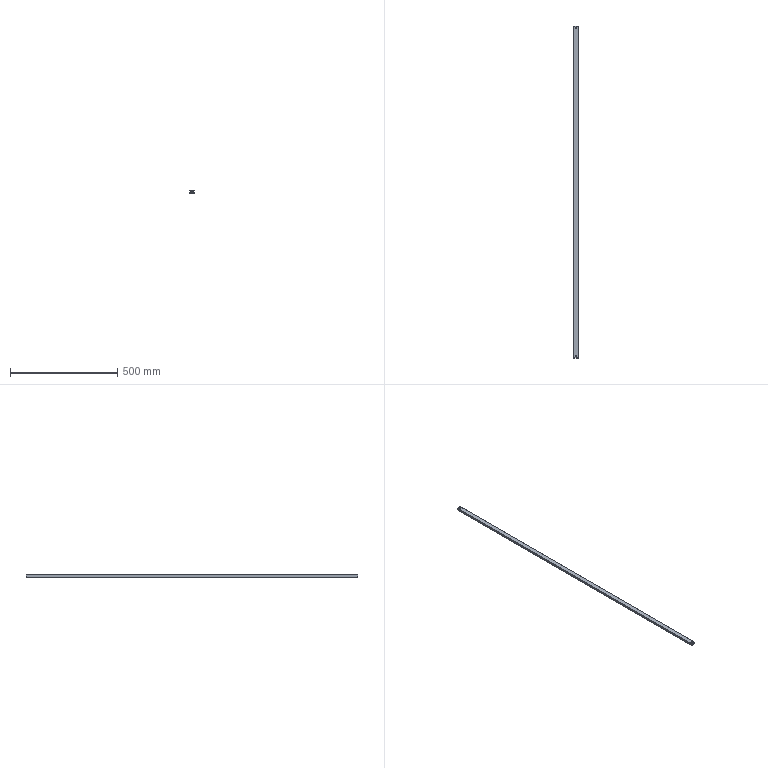Part | SolidWorks | features Extrusion 1, HoleWzd 1, WeldmentFeature 1 | 1 solid | 18 faces | box 20 x 1546 x 10 mm | volume 86388 mm3 | plane 10 | cylinder 8 | commonest cylinder face diameters 5.5 x4 10 x4
STEP:
#1=CARTESIAN_POINT('',(-5.,1538.3,-4.));
#2=VERTEX_POINT('',#1);
#3=CARTESIAN_POINT('',(5.,1538.3,-4.));
#4=VERTEX_POINT('',#3);
#5=CARTESIAN_POINT('',(0.,1538.3,-4.));
#6=DIRECTION('',(0.,0.,1.));
#7=DIRECTION('',(1.,0.,0.));
#8=AXIS2_PLACEMENT_3D('',#5,#6,#7);
#9=CIRCLE('',#8,5.);
#10=EDGE_CURVE('',#2,#4,#9,.T.);
#11=ORIENTED_EDGE('',*,*,#10,.T.);
#12=CARTESIAN_POINT('',(5.,1538.3,-5.));
#13=VERTEX_POINT('',#12);
#14=CARTESIAN_POINT('',(5.,1538.3,-5.));
#15=DIRECTION('',(0.,0.,-1.));
#16=VECTOR('',#15,1000.);
#17=LINE('',#14,#16);
#18=EDGE_CURVE('',#4,#13,#17,.T.);
#19=ORIENTED_EDGE('',*,*,#18,.T.);
#20=CARTESIAN_POINT('',(-5.,1538.3,-5.));
#21=VERTEX_POINT('',#20);
#22=CARTESIAN_POINT('',(0.,1538.3,-5.));
#23=DIRECTION('',(0.,0.,-1.));
#24=DIRECTION('',(-1.,0.,0.));
#25=AXIS2_PLACEMENT_3D('',#22,#23,#24);
#26=CIRCLE('',#25,5.);
#27=EDGE_CURVE('',#13,#21,#26,.T.);
#28=ORIENTED_EDGE('',*,*,#27,.T.);
#29=CARTESIAN_POINT('',(-5.,1538.3,-5.));
#30=DIRECTION('',(0.,0.,-1.));
#31=VECTOR('',#30,1000.);
#32=LINE('',#29,#31);
#33=EDGE_CURVE('',#2,#21,#32,.T.);
#34=ORIENTED_EDGE('',*,*,#33,.F.);
#35=EDGE_LOOP('',(#11,#19,#28,#34));
#36=FACE_OUTER_BOUND('',#35,.T.);
#37=CARTESIAN_POINT('',(0.,1538.3,-5.));
#38=DIRECTION('',(0.,0.,-1.));
#39=DIRECTION('',(-1.,0.,0.));
#40=AXIS2_PLACEMENT_3D('',#37,#38,#39);
#41=CYLINDRICAL_SURFACE('',#40,5.);
#42=ADVANCED_FACE('',(#36),#41,.F.);
#43=CARTESIAN_POINT('',(2.75,1538.3,5.));
#44=VERTEX_POINT('',#43);
#45=CARTESIAN_POINT('',(-2.75,1538.3,5.));
#46=VERTEX_POINT('',#45);
#47=CARTESIAN_POINT('',(0.,1538.3,5.));
#48=DIRECTION('',(0.,0.,-1.));
#49=DIRECTION('',(-1.,0.,0.));
#50=AXIS2_PLACEMENT_3D('',#47,#48,#49);
#51=CIRCLE('',#50,2.75);
#52=EDGE_CURVE('',#44,#46,#51,.T.);
#53=ORIENTED_EDGE('',*,*,#52,.F.);
#54=CARTESIAN_POINT('',(2.75,1538.3,4.));
#55=VERTEX_POINT('',#54);
#56=CARTESIAN_POINT('',(2.75,1538.3,-5.));
#57=DIRECTION('',(0.,0.,-1.));
#58=VECTOR('',#57,1000.);
#59=LINE('',#56,#58);
#60=EDGE_CURVE('',#44,#55,#59,.T.);
#61=ORIENTED_EDGE('',*,*,#60,.T.);
#62=CARTESIAN_POINT('',(-2.75,1538.3,4.));
#63=VERTEX_POINT('',#62);
#64=CARTESIAN_POINT('',(0.,1538.3,4.));
#65=DIRECTION('',(0.,0.,-1.));
#66=DIRECTION('',(-1.,0.,0.));
#67=AXIS2_PLACEMENT_3D('',#64,#65,#66);
#68=CIRCLE('',#67,2.75);
#69=EDGE_CURVE('',#55,#63,#68,.T.);
#70=ORIENTED_EDGE('',*,*,#69,.T.);
#71=CARTESIAN_POINT('',(-2.75,1538.3,-5.));
#72=DIRECTION('',(0.,0.,-1.));
#73=VECTOR('',#72,1000.);
#74=LINE('',#71,#73);
#75=EDGE_CURVE('',#46,#63,#74,.T.);
#76=ORIENTED_EDGE('',*,*,#75,.F.);
#77=EDGE_LOOP('',(#53,#61,#70,#76));
#78=FACE_OUTER_BOUND('',#77,.T.);
#79=CARTESIAN_POINT('',(0.,1538.3,-5.));
#80=DIRECTION('',(0.,0.,-1.));
#81=DIRECTION('',(-1.,0.,0.));
#82=AXIS2_PLACEMENT_3D('',#79,#80,#81);
#83=CYLINDRICAL_SURFACE('',#82,2.75);
#84=ADVANCED_FACE('',(#78),#83,.F.);
#85=CARTESIAN_POINT('',(2.75,8.,5.));
#86=VERTEX_POINT('',#85);
#87=CARTESIAN_POINT('',(-2.75,8.,5.));
#88=VERTEX_POINT('',#87);
#89=CARTESIAN_POINT('',(0.,8.,5.));
#90=DIRECTION('',(0.,0.,-1.));
#91=DIRECTION('',(-1.,0.,0.));
#92=AXIS2_PLACEMENT_3D('',#89,#90,#91);
#93=CIRCLE('',#92,2.75);
#94=EDGE_CURVE('',#86,#88,#93,.T.);
#95=ORIENTED_EDGE('',*,*,#94,.F.);
#96=CARTESIAN_POINT('',(2.75,8.,4.));
#97=VERTEX_POINT('',#96);
#98=CARTESIAN_POINT('',(2.75,8.,-5.));
#99=DIRECTION('',(0.,0.,-1.));
#100=VECTOR('',#99,1000.);
#101=LINE('',#98,#100);
#102=EDGE_CURVE('',#86,#97,#101,.T.);
#103=ORIENTED_EDGE('',*,*,#102,.T.);
#104=CARTESIAN_POINT('',(-2.75,8.,4.));
#105=VERTEX_POINT('',#104);
#106=CARTESIAN_POINT('',(0.,8.,4.));
#107=DIRECTION('',(0.,0.,-1.));
#108=DIRECTION('',(-1.,0.,0.));
#109=AXIS2_PLACEMENT_3D('',#106,#107,#108);
#110=CIRCLE('',#109,2.75);
#111=EDGE_CURVE('',#97,#105,#110,.T.);
#112=ORIENTED_EDGE('',*,*,#111,.T.);
#113=CARTESIAN_POINT('',(-2.75,8.,-5.));
#114=DIRECTION('',(0.,0.,-1.));
#115=VECTOR('',#114,1000.);
#116=LINE('',#113,#115);
#117=EDGE_CURVE('',#88,#105,#116,.T.);
#118=ORIENTED_EDGE('',*,*,#117,.F.);
#119=EDGE_LOOP('',(#95,#103,#112,#118));
#120=FACE_OUTER_BOUND('',#119,.T.);
#121=CARTESIAN_POINT('',(0.,8.,-5.));
#122=DIRECTION('',(0.,0.,-1.));
#123=DIRECTION('',(-1.,0.,0.));
#124=AXIS2_PLACEMENT_3D('',#121,#122,#123);
#125=CYLINDRICAL_SURFACE('',#124,2.75);
#126=ADVANCED_FACE('',(#120),#125,.F.);
#127=CARTESIAN_POINT('',(-5.,8.,-4.));
#128=VERTEX_POINT('',#127);
#129=CARTESIAN_POINT('',(5.,8.,-4.));
#130=VERTEX_POINT('',#129);
#131=CARTESIAN_POINT('',(0.,8.,-4.));
#132=DIRECTION('',(0.,0.,1.));
#133=DIRECTION('',(1.,0.,0.));
#134=AXIS2_PLACEMENT_3D('',#131,#132,#133);
#135=CIRCLE('',#134,5.);
#136=EDGE_CURVE('',#128,#130,#135,.T.);
#137=ORIENTED_EDGE('',*,*,#136,.T.);
#138=CARTESIAN_POINT('',(5.,8.,-5.));
#139=VERTEX_POINT('',#138);
#140=CARTESIAN_POINT('',(5.,8.,-5.));
#141=DIRECTION('',(0.,0.,-1.));
#142=VECTOR('',#141,1000.);
#143=LINE('',#140,#142);
#144=EDGE_CURVE('',#130,#139,#143,.T.);
#145=ORIENTED_EDGE('',*,*,#144,.T.);
#146=CARTESIAN_POINT('',(-5.,8.,-5.));
#147=VERTEX_POINT('',#146);
#148=CARTESIAN_POINT('',(0.,8.,-5.));
#149=DIRECTION('',(0.,0.,-1.));
#150=DIRECTION('',(-1.,0.,0.));
#151=AXIS2_PLACEMENT_3D('',#148,#149,#150);
#152=CIRCLE('',#151,5.);
#153=EDGE_CURVE('',#139,#147,#152,.T.);
#154=ORIENTED_EDGE('',*,*,#153,.T.);
#155=CARTESIAN_POINT('',(-5.,8.,-5.));
#156=DIRECTION('',(0.,0.,-1.));
#157=VECTOR('',#156,1000.);
#158=LINE('',#155,#157);
#159=EDGE_CURVE('',#128,#147,#158,.T.);
#160=ORIENTED_EDGE('',*,*,#159,.F.);
#161=EDGE_LOOP('',(#137,#145,#154,#160));
#162=FACE_OUTER_BOUND('',#161,.T.);
#163=CARTESIAN_POINT('',(0.,8.,-5.));
#164=DIRECTION('',(0.,0.,-1.));
#165=DIRECTION('',(-1.,0.,0.));
#166=AXIS2_PLACEMENT_3D('',#163,#164,#165);
#167=CYLINDRICAL_SURFACE('',#166,5.);
#168=ADVANCED_FACE('',(#162),#167,.F.);
#169=CARTESIAN_POINT('',(10.,1546.3,5.));
#170=VERTEX_POINT('',#169);
#171=CARTESIAN_POINT('',(10.,1546.3,-5.));
#172=VERTEX_POINT('',#171);
#173=CARTESIAN_POINT('',(10.,1546.3,-5.));
#174=DIRECTION('',(0.,0.,-1.));
#175=VECTOR('',#174,1000.);
#176=LINE('',#173,#175);
#177=EDGE_CURVE('',#170,#172,#176,.T.);
#178=ORIENTED_EDGE('',*,*,#177,.T.);
#179=CARTESIAN_POINT('',(-10.,1546.3,-5.));
#180=VERTEX_POINT('',#179);
#181=CARTESIAN_POINT('',(-10.,1546.3,-5.));
#182=DIRECTION('',(-1.,0.,0.));
#183=VECTOR('',#182,1000.);
#184=LINE('',#181,#183);
#185=EDGE_CURVE('',#172,#180,#184,.T.);
#186=ORIENTED_EDGE('',*,*,#185,.T.);
#187=CARTESIAN_POINT('',(-10.,1546.3,5.));
#188=VERTEX_POINT('',#187);
#189=CARTESIAN_POINT('',(-10.,1546.3,-5.));
#190=DIRECTION('',(0.,0.,1.));
#191=VECTOR('',#190,1000.);
#192=LINE('',#189,#191);
#193=EDGE_CURVE('',#180,#188,#192,.T.);
#194=ORIENTED_EDGE('',*,*,#193,.T.);
#195=CARTESIAN_POINT('',(-10.,1546.3,5.));
#196=DIRECTION('',(1.,0.,0.));
#197=VECTOR('',#196,1000.);
#198=LINE('',#195,#197);
#199=EDGE_CURVE('',#188,#170,#198,.T.);
#200=ORIENTED_EDGE('',*,*,#199,.T.);
#201=EDGE_LOOP('',(#178,#186,#194,#200));
#202=FACE_OUTER_BOUND('',#201,.T.);
#203=CARTESIAN_POINT('',(-9.,1546.3,-4.));
#204=VERTEX_POINT('',#203);
#205=CARTESIAN_POINT('',(-9.,1546.3,4.));
#206=VERTEX_POINT('',#205);
#207=CARTESIAN_POINT('',(-9.,1546.3,-4.));
#208=DIRECTION('',(0.,0.,1.));
#209=VECTOR('',#208,1000.);
#210=LINE('',#207,#209);
#211=EDGE_CURVE('',#204,#206,#210,.T.);
#212=ORIENTED_EDGE('',*,*,#211,.F.);
#213=CARTESIAN_POINT('',(9.,1546.3,-4.));
#214=VERTEX_POINT('',#213);
#215=CARTESIAN_POINT('',(-9.,1546.3,-4.));
#216=DIRECTION('',(-1.,0.,0.));
#217=VECTOR('',#216,1000.);
#218=LINE('',#215,#217);
#219=EDGE_CURVE('',#214,#204,#218,.T.);
#220=ORIENTED_EDGE('',*,*,#219,.F.);
#221=CARTESIAN_POINT('',(9.,1546.3,4.));
#222=VERTEX_POINT('',#221);
#223=CARTESIAN_POINT('',(9.,1546.3,-4.));
#224=DIRECTION('',(0.,0.,-1.));
#225=VECTOR('',#224,1000.);
#226=LINE('',#223,#225);
#227=EDGE_CURVE('',#222,#214,#226,.T.);
#228=ORIENTED_EDGE('',*,*,#227,.F.);
#229=CARTESIAN_POINT('',(-9.,1546.3,4.));
#230=DIRECTION('',(1.,0.,0.));
#231=VECTOR('',#230,1000.);
#232=LINE('',#229,#231);
#233=EDGE_CURVE('',#206,#222,#232,.T.);
#234=ORIENTED_EDGE('',*,*,#233,.F.);
#235=EDGE_LOOP('',(#212,#220,#228,#234));
#236=FACE_BOUND('',#235,.T.);
#237=CARTESIAN_POINT('',(0.,1546.3,0.));
#238=DIRECTION('',(0.,1.,0.));
#239=DIRECTION('',(0.,0.,1.));
#240=AXIS2_PLACEMENT_3D('',#237,#238,#239);
#241=PLANE('',#240);
#242=ADVANCED_FACE('',(#202,#236),#241,.T.);
#243=CARTESIAN_POINT('',(10.,0.,5.));
#244=VERTEX_POINT('',#243);
#245=CARTESIAN_POINT('',(10.,0.,-5.));
#246=VERTEX_POINT('',#245);
#247=CARTESIAN_POINT('',(10.,0.,-5.));
#248=DIRECTION('',(0.,0.,-1.));
#249=VECTOR('',#248,1000.);
#250=LINE('',#247,#249);
#251=EDGE_CURVE('',#244,#246,#250,.T.);
#252=ORIENTED_EDGE('',*,*,#251,.F.);
#253=CARTESIAN_POINT('',(-10.,0.,5.));
#254=VERTEX_POINT('',#253);
#255=CARTESIAN_POINT('',(-10.,0.,5.));
#256=DIRECTION('',(1.,0.,0.));
#257=VECTOR('',#256,1000.);
#258=LINE('',#255,#257);
#259=EDGE_CURVE('',#254,#244,#258,.T.);
#260=ORIENTED_EDGE('',*,*,#259,.F.);
#261=CARTESIAN_POINT('',(-10.,0.,-5.));
#262=VERTEX_POINT('',#261);
#263=CARTESIAN_POINT('',(-10.,0.,-5.));
#264=DIRECTION('',(0.,0.,1.));
#265=VECTOR('',#264,1000.);
#266=LINE('',#263,#265);
#267=EDGE_CURVE('',#262,#254,#266,.T.);
#268=ORIENTED_EDGE('',*,*,#267,.F.);
#269=CARTESIAN_POINT('',(-10.,0.,-5.));
#270=DIRECTION('',(-1.,0.,0.));
#271=VECTOR('',#270,1000.);
#272=LINE('',#269,#271);
#273=EDGE_CURVE('',#246,#262,#272,.T.);
#274=ORIENTED_EDGE('',*,*,#273,.F.);
#275=EDGE_LOOP('',(#252,#260,#268,#274));
#276=FACE_OUTER_BOUND('',#275,.T.);
#277=CARTESIAN_POINT('',(9.,0.,-4.));
#278=VERTEX_POINT('',#277);
#279=CARTESIAN_POINT('',(-9.,0.,-4.));
#280=VERTEX_POINT('',#279);
#281=CARTESIAN_POINT('',(-9.,0.,-4.));
#282=DIRECTION('',(-1.,0.,0.));
#283=VECTOR('',#282,1000.);
#284=LINE('',#281,#283);
#285=EDGE_CURVE('',#278,#280,#284,.T.);
#286=ORIENTED_EDGE('',*,*,#285,.T.);
#287=CARTESIAN_POINT('',(-9.,0.,4.));
#288=VERTEX_POINT('',#287);
#289=CARTESIAN_POINT('',(-9.,0.,-4.));
#290=DIRECTION('',(0.,0.,1.));
#291=VECTOR('',#290,1000.);
#292=LINE('',#289,#291);
#293=EDGE_CURVE('',#280,#288,#292,.T.);
#294=ORIENTED_EDGE('',*,*,#293,.T.);
#295=CARTESIAN_POINT('',(9.,0.,4.));
#296=VERTEX_POINT('',#295);
#297=CARTESIAN_POINT('',(-9.,0.,4.));
#298=DIRECTION('',(1.,0.,0.));
#299=VECTOR('',#298,1000.);
#300=LINE('',#297,#299);
#301=EDGE_CURVE('',#288,#296,#300,.T.);
#302=ORIENTED_EDGE('',*,*,#301,.T.);
#303=CARTESIAN_POINT('',(9.,0.,-4.));
#304=DIRECTION('',(0.,0.,-1.));
#305=VECTOR('',#304,1000.);
#306=LINE('',#303,#305);
#307=EDGE_CURVE('',#296,#278,#306,.T.);
#308=ORIENTED_EDGE('',*,*,#307,.T.);
#309=EDGE_LOOP('',(#286,#294,#302,#308));
#310=FACE_BOUND('',#309,.T.);
#311=CARTESIAN_POINT('',(0.,0.,0.));
#312=DIRECTION('',(0.,1.,0.));
#313=DIRECTION('',(0.,0.,1.));
#314=AXIS2_PLACEMENT_3D('',#311,#312,#313);
#315=PLANE('',#314);
#316=ADVANCED_FACE('',(#276,#310),#315,.F.);
#317=ORIENTED_EDGE('',*,*,#251,.T.);
#318=CARTESIAN_POINT('',(10.,1546.3,-5.));
#319=DIRECTION('',(0.,-1.,0.));
#320=VECTOR('',#319,1000.);
#321=LINE('',#318,#320);
#322=EDGE_CURVE('',#172,#246,#321,.T.);
#323=ORIENTED_EDGE('',*,*,#322,.F.);
#324=ORIENTED_EDGE('',*,*,#177,.F.);
#325=CARTESIAN_POINT('',(10.,1546.3,5.));
#326=DIRECTION('',(0.,-1.,0.));
#327=VECTOR('',#326,1000.);
#328=LINE('',#325,#327);
#329=EDGE_CURVE('',#170,#244,#328,.T.);
#330=ORIENTED_EDGE('',*,*,#329,.T.);
#331=EDGE_LOOP('',(#317,#323,#324,#330));
#332=FACE_OUTER_BOUND('',#331,.T.);
#333=CARTESIAN_POINT('',(10.,1546.3,-5.));
#334=DIRECTION('',(-1.,0.,0.));
#335=DIRECTION('',(0.,0.,1.));
#336=AXIS2_PLACEMENT_3D('',#333,#334,#335);
#337=PLANE('',#336);
#338=ADVANCED_FACE('',(#332),#337,.F.);
#339=CARTESIAN_POINT('',(0.,1538.3,-5.));
#340=DIRECTION('',(0.,0.,-1.));
#341=DIRECTION('',(-1.,0.,0.));
#342=AXIS2_PLACEMENT_3D('',#339,#340,#341);
#343=CIRCLE('',#342,5.);
#344=EDGE_CURVE('',#21,#13,#343,.T.);
#345=ORIENTED_EDGE('',*,*,#344,.F.);
#346=ORIENTED_EDGE('',*,*,#27,.F.);
#347=EDGE_LOOP('',(#345,#346));
#348=FACE_BOUND('',#347,.T.);
#349=CARTESIAN_POINT('',(0.,8.,-5.));
#350=DIRECTION('',(0.,0.,-1.));
#351=DIRECTION('',(-1.,0.,0.));
#352=AXIS2_PLACEMENT_3D('',#349,#350,#351);
#353=CIRCLE('',#352,5.);
#354=EDGE_CURVE('',#147,#139,#353,.T.);
#355=ORIENTED_EDGE('',*,*,#354,.F.);
#356=ORIENTED_EDGE('',*,*,#153,.F.);
#357=EDGE_LOOP('',(#355,#356));
#358=FACE_BOUND('',#357,.T.);
#359=ORIENTED_EDGE('',*,*,#273,.T.);
#360=CARTESIAN_POINT('',(-10.,1546.3,-5.));
#361=DIRECTION('',(0.,-1.,0.));
#362=VECTOR('',#361,1000.);
#363=LINE('',#360,#362);
#364=EDGE_CURVE('',#180,#262,#363,.T.);
#365=ORIENTED_EDGE('',*,*,#364,.F.);
#366=ORIENTED_EDGE('',*,*,#185,.F.);
#367=ORIENTED_EDGE('',*,*,#322,.T.);
#368=EDGE_LOOP('',(#359,#365,#366,#367));
#369=FACE_OUTER_BOUND('',#368,.T.);
#370=CARTESIAN_POINT('',(-10.,1546.3,-5.));
#371=DIRECTION('',(0.,0.,1.));
#372=DIRECTION('',(1.,0.,0.));
#373=AXIS2_PLACEMENT_3D('',#370,#371,#372);
#374=PLANE('',#373);
#375=ADVANCED_FACE('',(#348,#358,#369),#374,.F.);
#376=ORIENTED_EDGE('',*,*,#267,.T.);
#377=CARTESIAN_POINT('',(-10.,1546.3,5.));
#378=DIRECTION('',(0.,-1.,0.));
#379=VECTOR('',#378,1000.);
#380=LINE('',#377,#379);
#381=EDGE_CURVE('',#188,#254,#380,.T.);
#382=ORIENTED_EDGE('',*,*,#381,.F.);
#383=ORIENTED_EDGE('',*,*,#193,.F.);
#384=ORIENTED_EDGE('',*,*,#364,.T.);
#385=EDGE_LOOP('',(#376,#382,#383,#384));
#386=FACE_OUTER_BOUND('',#385,.T.);
#387=CARTESIAN_POINT('',(-10.,1546.3,-5.));
#388=DIRECTION('',(1.,0.,0.));
#389=DIRECTION('',(0.,0.,-1.));
#390=AXIS2_PLACEMENT_3D('',#387,#388,#389);
#391=PLANE('',#390);
#392=ADVANCED_FACE('',(#386),#391,.F.);
#393=CARTESIAN_POINT('',(0.,1538.3,5.));
#394=DIRECTION('',(0.,0.,-1.));
#395=DIRECTION('',(-1.,0.,0.));
#396=AXIS2_PLACEMENT_3D('',#393,#394,#395);
#397=CIRCLE('',#396,2.75);
#398=EDGE_CURVE('',#46,#44,#397,.T.);
#399=ORIENTED_EDGE('',*,*,#398,.T.);
#400=ORIENTED_EDGE('',*,*,#52,.T.);
#401=EDGE_LOOP('',(#399,#400));
#402=FACE_BOUND('',#401,.T.);
#403=CARTESIAN_POINT('',(0.,8.,5.));
#404=DIRECTION('',(0.,0.,-1.));
#405=DIRECTION('',(-1.,0.,0.));
#406=AXIS2_PLACEMENT_3D('',#403,#404,#405);
#407=CIRCLE('',#406,2.75);
#408=EDGE_CURVE('',#88,#86,#407,.T.);
#409=ORIENTED_EDGE('',*,*,#408,.T.);
#410=ORIENTED_EDGE('',*,*,#94,.T.);
#411=EDGE_LOOP('',(#409,#410));
#412=FACE_BOUND('',#411,.T.);
#413=ORIENTED_EDGE('',*,*,#259,.T.);
#414=ORIENTED_EDGE('',*,*,#329,.F.);
#415=ORIENTED_EDGE('',*,*,#199,.F.);
#416=ORIENTED_EDGE('',*,*,#381,.T.);
#417=EDGE_LOOP('',(#413,#414,#415,#416));
#418=FACE_OUTER_BOUND('',#417,.T.);
#419=CARTESIAN_POINT('',(-10.,1546.3,5.));
#420=DIRECTION('',(0.,0.,-1.));
#421=DIRECTION('',(-1.,0.,0.));
#422=AXIS2_PLACEMENT_3D('',#419,#420,#421);
#423=PLANE('',#422);
#424=ADVANCED_FACE('',(#402,#412,#418),#423,.F.);
#425=ORIENTED_EDGE('',*,*,#10,.F.);
#426=CARTESIAN_POINT('',(0.,1538.3,-4.));
#427=DIRECTION('',(0.,0.,1.));
#428=DIRECTION('',(1.,0.,0.));
#429=AXIS2_PLACEMENT_3D('',#426,#427,#428);
#430=CIRCLE('',#429,5.);
#431=EDGE_CURVE('',#4,#2,#430,.T.);
#432=ORIENTED_EDGE('',*,*,#431,.F.);
#433=EDGE_LOOP('',(#425,#432));
#434=FACE_BOUND('',#433,.T.);
#435=ORIENTED_EDGE('',*,*,#136,.F.);
#436=CARTESIAN_POINT('',(0.,8.,-4.));
#437=DIRECTION('',(0.,0.,1.));
#438=DIRECTION('',(1.,0.,0.));
#439=AXIS2_PLACEMENT_3D('',#436,#437,#438);
#440=CIRCLE('',#439,5.);
#441=EDGE_CURVE('',#130,#128,#440,.T.);
#442=ORIENTED_EDGE('',*,*,#441,.F.);
#443=EDGE_LOOP('',(#435,#442));
#444=FACE_BOUND('',#443,.T.);
#445=ORIENTED_EDGE('',*,*,#285,.F.);
#446=CARTESIAN_POINT('',(9.,1546.3,-4.));
#447=DIRECTION('',(0.,-1.,0.));
#448=VECTOR('',#447,1000.);
#449=LINE('',#446,#448);
#450=EDGE_CURVE('',#214,#278,#449,.T.);
#451=ORIENTED_EDGE('',*,*,#450,.F.);
#452=ORIENTED_EDGE('',*,*,#219,.T.);
#453=CARTESIAN_POINT('',(-9.,1546.3,-4.));
#454=DIRECTION('',(0.,-1.,0.));
#455=VECTOR('',#454,1000.);
#456=LINE('',#453,#455);
#457=EDGE_CURVE('',#204,#280,#456,.T.);
#458=ORIENTED_EDGE('',*,*,#457,.T.);
#459=EDGE_LOOP('',(#445,#451,#452,#458));
#460=FACE_OUTER_BOUND('',#459,.T.);
#461=CARTESIAN_POINT('',(-9.,1546.3,-4.));
#462=DIRECTION('',(0.,0.,1.));
#463=DIRECTION('',(1.,0.,0.));
#464=AXIS2_PLACEMENT_3D('',#461,#462,#463);
#465=PLANE('',#464);
#466=ADVANCED_FACE('',(#434,#444,#460),#465,.T.);
#467=ORIENTED_EDGE('',*,*,#293,.F.);
#468=ORIENTED_EDGE('',*,*,#457,.F.);
#469=ORIENTED_EDGE('',*,*,#211,.T.);
#470=CARTESIAN_POINT('',(-9.,1546.3,4.));
#471=DIRECTION('',(0.,-1.,0.));
#472=VECTOR('',#471,1000.);
#473=LINE('',#470,#472);
#474=EDGE_CURVE('',#206,#288,#473,.T.);
#475=ORIENTED_EDGE('',*,*,#474,.T.);
#476=EDGE_LOOP('',(#467,#468,#469,#475));
#477=FACE_OUTER_BOUND('',#476,.T.);
#478=CARTESIAN_POINT('',(-9.,1546.3,-4.));
#479=DIRECTION('',(1.,0.,0.));
#480=DIRECTION('',(0.,0.,-1.));
#481=AXIS2_PLACEMENT_3D('',#478,#479,#480);
#482=PLANE('',#481);
#483=ADVANCED_FACE('',(#477),#482,.T.);
#484=CARTESIAN_POINT('',(0.,1538.3,4.));
#485=DIRECTION('',(0.,0.,-1.));
#486=DIRECTION('',(-1.,0.,0.));
#487=AXIS2_PLACEMENT_3D('',#484,#485,#486);
#488=CIRCLE('',#487,2.75);
#489=EDGE_CURVE('',#63,#55,#488,.T.);
#490=ORIENTED_EDGE('',*,*,#489,.F.);
#491=ORIENTED_EDGE('',*,*,#69,.F.);
#492=EDGE_LOOP('',(#490,#491));
#493=FACE_BOUND('',#492,.T.);
#494=CARTESIAN_POINT('',(0.,8.,4.));
#495=DIRECTION('',(0.,0.,-1.));
#496=DIRECTION('',(-1.,0.,0.));
#497=AXIS2_PLACEMENT_3D('',#494,#495,#496);
#498=CIRCLE('',#497,2.75);
#499=EDGE_CURVE('',#105,#97,#498,.T.);
#500=ORIENTED_EDGE('',*,*,#499,.F.);
#501=ORIENTED_EDGE('',*,*,#111,.F.);
#502=EDGE_LOOP('',(#500,#501));
#503=FACE_BOUND('',#502,.T.);
#504=ORIENTED_EDGE('',*,*,#301,.F.);
#505=ORIENTED_EDGE('',*,*,#474,.F.);
#506=ORIENTED_EDGE('',*,*,#233,.T.);
#507=CARTESIAN_POINT('',(9.,1546.3,4.));
#508=DIRECTION('',(0.,-1.,0.));
#509=VECTOR('',#508,1000.);
#510=LINE('',#507,#509);
#511=EDGE_CURVE('',#222,#296,#510,.T.);
#512=ORIENTED_EDGE('',*,*,#511,.T.);
#513=EDGE_LOOP('',(#504,#505,#506,#512));
#514=FACE_OUTER_BOUND('',#513,.T.);
#515=CARTESIAN_POINT('',(-9.,1546.3,4.));
#516=DIRECTION('',(0.,0.,-1.));
#517=DIRECTION('',(-1.,0.,0.));
#518=AXIS2_PLACEMENT_3D('',#515,#516,#517);
#519=PLANE('',#518);
#520=ADVANCED_FACE('',(#493,#503,#514),#519,.T.);
#521=ORIENTED_EDGE('',*,*,#307,.F.);
#522=ORIENTED_EDGE('',*,*,#511,.F.);
#523=ORIENTED_EDGE('',*,*,#227,.T.);
#524=ORIENTED_EDGE('',*,*,#450,.T.);
#525=EDGE_LOOP('',(#521,#522,#523,#524));
#526=FACE_OUTER_BOUND('',#525,.T.);
#527=CARTESIAN_POINT('',(9.,1546.3,-4.));
#528=DIRECTION('',(-1.,0.,0.));
#529=DIRECTION('',(0.,0.,1.));
#530=AXIS2_PLACEMENT_3D('',#527,#528,#529);
#531=PLANE('',#530);
#532=ADVANCED_FACE('',(#526),#531,.T.);
#533=ORIENTED_EDGE('',*,*,#144,.F.);
#534=ORIENTED_EDGE('',*,*,#441,.T.);
#535=ORIENTED_EDGE('',*,*,#159,.T.);
#536=ORIENTED_EDGE('',*,*,#354,.T.);
#537=EDGE_LOOP('',(#533,#534,#535,#536));
#538=FACE_OUTER_BOUND('',#537,.T.);
#539=CARTESIAN_POINT('',(0.,8.,-5.));
#540=DIRECTION('',(0.,0.,-1.));
#541=DIRECTION('',(-1.,0.,0.));
#542=AXIS2_PLACEMENT_3D('',#539,#540,#541);
#543=CYLINDRICAL_SURFACE('',#542,5.);
#544=ADVANCED_FACE('',(#538),#543,.F.);
#545=ORIENTED_EDGE('',*,*,#102,.F.);
#546=ORIENTED_EDGE('',*,*,#408,.F.);
#547=ORIENTED_EDGE('',*,*,#117,.T.);
#548=ORIENTED_EDGE('',*,*,#499,.T.);
#549=EDGE_LOOP('',(#545,#546,#547,#548));
#550=FACE_OUTER_BOUND('',#549,.T.);
#551=CARTESIAN_POINT('',(0.,8.,-5.));
#552=DIRECTION('',(0.,0.,-1.));
#553=DIRECTION('',(-1.,0.,0.));
#554=AXIS2_PLACEMENT_3D('',#551,#552,#553);
#555=CYLINDRICAL_SURFACE('',#554,2.75);
#556=ADVANCED_FACE('',(#550),#555,.F.);
#557=ORIENTED_EDGE('',*,*,#60,.F.);
#558=ORIENTED_EDGE('',*,*,#398,.F.);
#559=ORIENTED_EDGE('',*,*,#75,.T.);
#560=ORIENTED_EDGE('',*,*,#489,.T.);
#561=EDGE_LOOP('',(#557,#558,#559,#560));
#562=FACE_OUTER_BOUND('',#561,.T.);
#563=CARTESIAN_POINT('',(0.,1538.3,-5.));
#564=DIRECTION('',(0.,0.,-1.));
#565=DIRECTION('',(-1.,0.,0.));
#566=AXIS2_PLACEMENT_3D('',#563,#564,#565);
#567=CYLINDRICAL_SURFACE('',#566,2.75);
#568=ADVANCED_FACE('',(#562),#567,.F.);
#569=ORIENTED_EDGE('',*,*,#18,.F.);
#570=ORIENTED_EDGE('',*,*,#431,.T.);
#571=ORIENTED_EDGE('',*,*,#33,.T.);
#572=ORIENTED_EDGE('',*,*,#344,.T.);
#573=EDGE_LOOP('',(#569,#570,#571,#572));
#574=FACE_OUTER_BOUND('',#573,.T.);
#575=CARTESIAN_POINT('',(0.,1538.3,-5.));
#576=DIRECTION('',(0.,0.,-1.));
#577=DIRECTION('',(-1.,0.,0.));
#578=AXIS2_PLACEMENT_3D('',#575,#576,#577);
#579=CYLINDRICAL_SURFACE('',#578,5.);
#580=ADVANCED_FACE('',(#574),#579,.F.);
#581=CLOSED_SHELL('',(#42,#84,#126,#168,#242,#316,#338,#375,#392,#424,#466,#483,#520,#532,#544,#556,#568,#580));
#582=MANIFOLD_SOLID_BREP('',#581);
#583=CARTESIAN_POINT('',(0.,0.,0.));
#584=DIRECTION('',(0.,0.,1.));
#585=DIRECTION('',(1.,0.,0.));
#586=AXIS2_PLACEMENT_3D('',#583,#584,#585);
#587=(LENGTH_UNIT()NAMED_UNIT(*)SI_UNIT(.MILLI.,.METRE.));
#588=UNCERTAINTY_MEASURE_WITH_UNIT(LENGTH_MEASURE(0.00001),#587,'','');
#589=(NAMED_UNIT(*)PLANE_ANGLE_UNIT()SI_UNIT($,.RADIAN.));
#590=(NAMED_UNIT(*)SI_UNIT($,.STERADIAN.)SOLID_ANGLE_UNIT());
#591=(GEOMETRIC_REPRESENTATION_CONTEXT(3)GLOBAL_UNCERTAINTY_ASSIGNED_CONTEXT((#588))GLOBAL_UNIT_ASSIGNED_CONTEXT((#587,#589,#590))REPRESENTATION_CONTEXT('',''));
#592=ADVANCED_BREP_SHAPE_REPRESENTATION('',(#582,#586),#591);